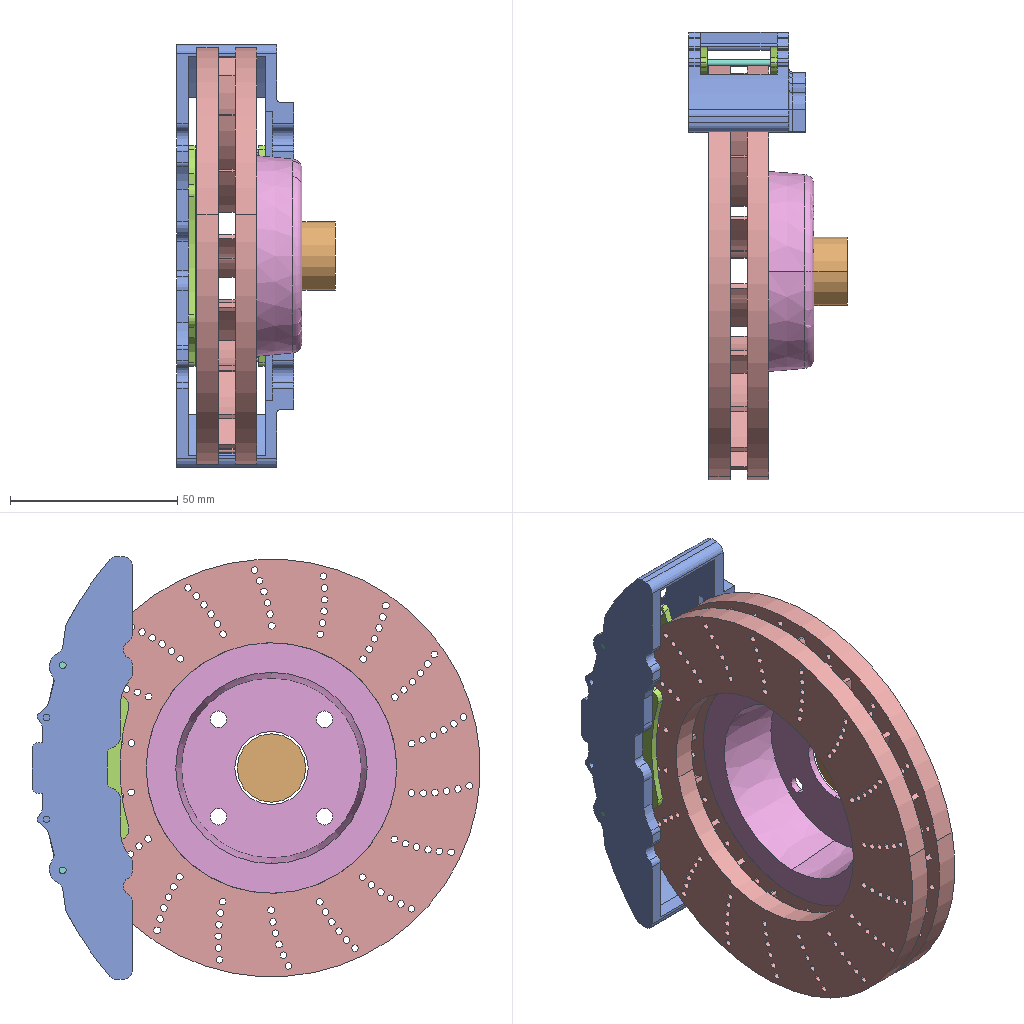Assembly | SolidWorks | 5 different items | 6 placed | box 47 x 134 x 127 mm
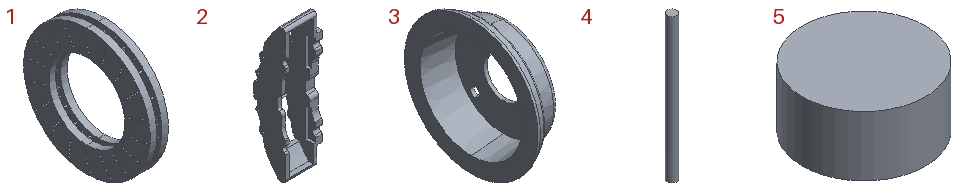Parts list (item | quantity | size | volume | features):
1 | x1 | 18 x 125 x 125 mm | 100342 mm3 | features CirPattern 2, Fillet 2, ICE 2, BossThin 1, CurvePattern 1, Extrusion 1, MirrorPattern 1
2 | x1 | 35 x 30 x 126.513 mm | 25595 mm3 | features ICE 6, Fillet 2, Extrusion 1, Shell 1
3 | x1 | 20 x 75 x 75 mm | 17771 mm3 | features Fillet 2, ICE 1, Revolution 1
4 | x2 | 2 x 2 x 30 mm | 94.248 mm3 | features Extrusion 1
5 | x1 | 20.49 x 20.49 x 10 mm | 3298 mm3 | features Extrusion 1
Mates (type | each side: item.copy, entity, surface, feature):
Concentric | 1.1 face cylinder Mirror1 | 3.1 face cylinder Revolve1
Coincident | 1.1 edge | 3.1 face plane Revolve1
Concentric | 3.1 edge | assembly select_type:10
Concentric | 2.1 face cylinder Cut-Extrude1 | 4.1 face cylinder Boss-Extrude1
Coincident | 2.1 face plane Boss-Extrude1 | 4.1 face plane Boss-Extrude1
Concentric | 2.1 face cylinder Cut-Extrude1 | 4.2 face cylinder Boss-Extrude1
Coincident | 2.1 face plane Boss-Extrude1 | 4.2 face plane Boss-Extrude1